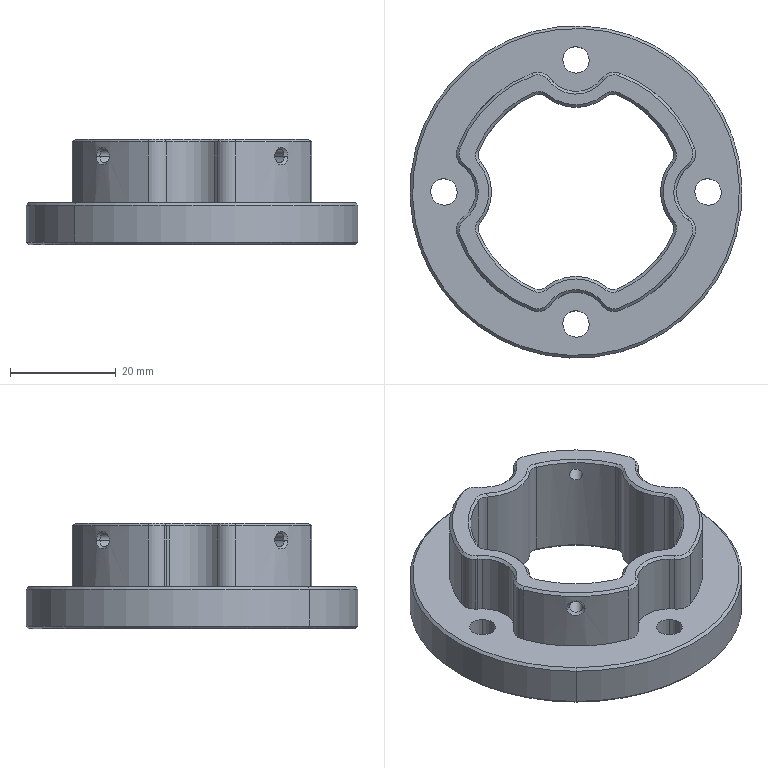NC program | NX | posted with a generic post | part box 62.9 x 62.9 x 20 mm
Lines 7601 to 7695 of 7695:
(DRILLING , TOOL : D6A45)
N15164 T01 M6
N15166 G54
N15168 G17 G0 G90 X0. Y-25. S5000 M3
N15170 G43 Z30. H1
N15172 G94 G81 G98 Z-14.6 F350. R-9.
N15174 X-25. Y0.
N15176 X0. Y25.
N15178 X25. Y0.
N15180 G80
N15182 G0 X25. Y0. Z30.
N15184 M5
(DRILLING_COPY_1_COPY , TOOL : 5.0ZT)
N15186 T05 M6
N15188 G54
N15190 G17 G0 G90 X0. Y-25. S2000 M3
N15192 G43 Z30. H5
N15194 G94 G83 G98 Z-23.002 F200. Q2. R-9.
N15196 X-25. Y0.
N15198 X0. Y25.
N15200 X25. Y0.
N15202 G80
N15204 G0 X25. Y0. Z30.
N15206 M5
(PLANAR_MILL_COPY_COPY_COPY_COPY_COPY_COPY_1 , TOOL : D6A45)
N15208 T01 M6
N15210 G54
N15212 G17 G0 G90 X-4.106 Y22.964 S9500 M3
N15214 G43 Z30. H1
N15216 Z0.
N15218 G94 G1 Z-1.5 F1250.
N15220 G3 X-3.979 Y21.972 R1.
N15222 X4.024 Y22.032 R5.
N15224 G2 X8.626 Y23.411 R4.
N15226 X23.411 Y8.626 R24.95
N15228 X22.032 Y4.024 R4.
N15230 G3 X22.032 Y-4.024 R5.
N15232 G2 X23.411 Y-8.626 R4.
N15234 X8.626 Y-23.411 R24.95
N15236 X4.024 Y-22.032 R4.
N15238 G3 X-4.024 Y-22.032 R5.
N15240 G2 X-8.626 Y-23.411 R4.
N15242 X-23.411 Y-8.626 R24.95
N15244 X-22.032 Y-4.024 R4.
N15246 G3 X-22.032 Y4.024 R5.
N15248 G2 X-23.411 Y8.626 R4.
N15250 X-8.626 Y23.411 R24.95
N15252 X-3.979 Y21.972 R4.001
N15254 G3 X-3.057 Y21.586 R1.
N15256 G1 Z0.
N15258 G0 Z30.
N15260 X0.866 Y14.5
N15262 Z0.
N15264 G1 Z-1.5
N15266 G3 X0. Y15. R1.
N15268 G2 X-6.374 Y17.295 R10.
N15270 G3 X-7.402 Y17.445 R1.
N15272 X-17.445 Y7.402 R18.95
N15274 X-17.295 Y6.374 R1.
N15276 G2 X-17.295 Y-6.374 R10.
N15278 G3 X-17.445 Y-7.402 R1.
N15280 X-7.402 Y-17.445 R18.95
N15282 X-6.374 Y-17.295 R1.
N15284 G2 X6.374 Y-17.295 R10.
N15286 G3 X7.402 Y-17.445 R1.
N15288 X17.445 Y-7.402 R18.95
N15290 X17.295 Y-6.374 R1.
N15292 G2 X17.295 Y6.374 R10.
N15294 G3 X17.445 Y7.402 R1.
N15296 X7.402 Y17.445 R18.95
N15298 X6.374 Y17.295 R1.
N15300 G2 X0. Y15. R10.
N15302 G3 X-0.866 Y14.5 R1.
N15304 G1 Z0.
N15306 G0 Z30.
(PLANAR_MILL_COPY_COPY_COPY_COPY_COPY_COPY_1_COPY , TOOL : D6A45)
N15308 X-22.687 Y-23.912
N15310 Z-12.
N15312 G1 Z-13.5
N15314 G3 X-22.946 Y-22.946 R1.
N15316 G2 X-22.946 Y22.946 R32.45
N15318 X-22.946 Y-22.946 R-32.45
N15320 G3 X-23.912 Y-22.687 R1.
N15322 G1 Z-12.
N15324 G0 Z30.
N15326 M5
N15328 M2